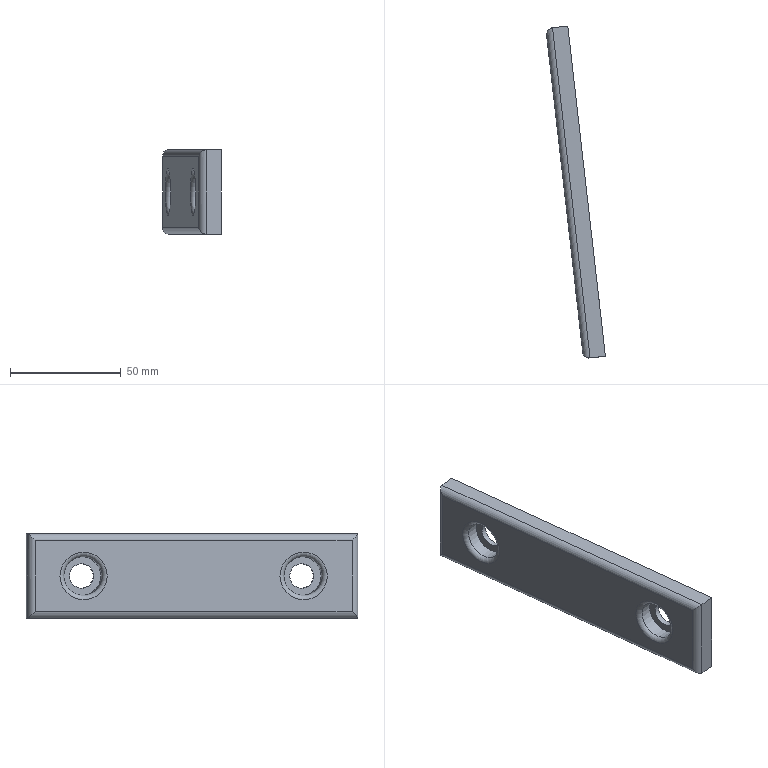Part | NX | features DB 2 | 1 solid | 148 faces | box 26.596 x 149.847 x 38 mm | volume 52095 mm3 | plane 97 | spline 41 | cylinder 8 | torus 2 | commonest cylinder face diameters 6 x4 11 x2 17.5 x2